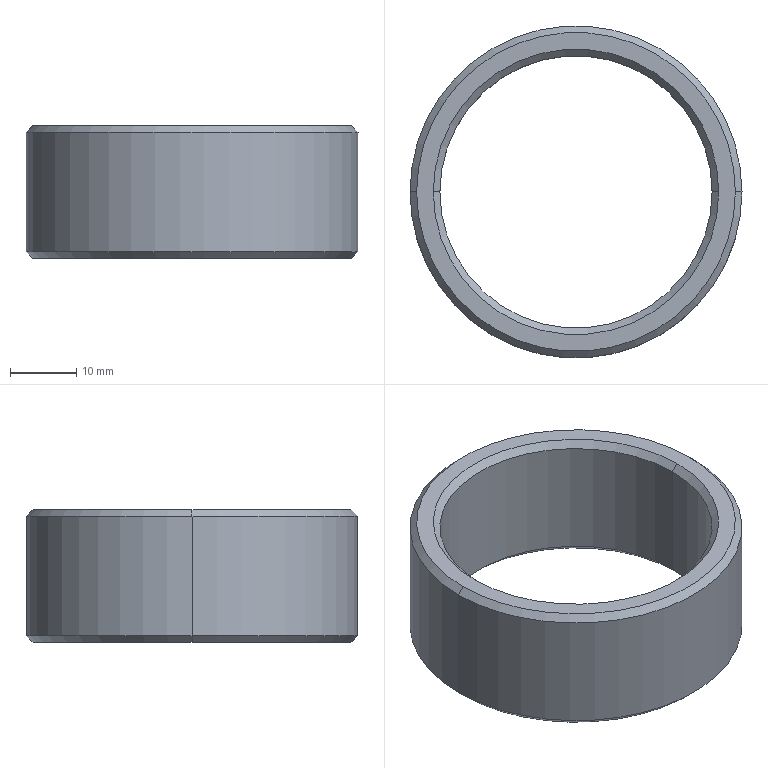Part | STEP file | 1 solid | 14 faces | box 50 x 50 x 20 mm | volume 12579 mm3 | cone 8 | cylinder 4 | plane 2 | commonest cylinder face diameters 41 x2 50 x2
STEP:
#1=CARTESIAN_POINT('',(0.,0.,0.));
#2=DIRECTION('',(0.,0.,1.));
#3=DIRECTION('',(1.,0.,0.));
#4=AXIS2_PLACEMENT_3D('',#1,#2,#3);
#5=CARTESIAN_POINT('',(-20.5,0.,1.));
#6=VERTEX_POINT('',#5);
#7=CARTESIAN_POINT('',(20.5,0.,1.));
#8=VERTEX_POINT('',#7);
#9=CARTESIAN_POINT('',(0.,0.,1.));
#10=DIRECTION('',(0.,0.,-1.));
#11=DIRECTION('',(-1.,0.,0.));
#12=AXIS2_PLACEMENT_3D('',#9,#10,#11);
#13=CIRCLE('',#12,20.5);
#14=CARTESIAN_POINT('',(0.,0.,20.));
#15=DIRECTION('',(0.,0.,-1.));
#16=DIRECTION('',(-1.,0.,0.));
#17=AXIS2_PLACEMENT_3D('',#14,#15,#16);
#18=CYLINDRICAL_SURFACE('',#17,20.5);
#19=CARTESIAN_POINT('',(0.,19.));
#20=DIRECTION('',(1.,0.));
#21=VECTOR('',#20,1.);
#22=LINE('',#19,#21);
#23=(GEOMETRIC_REPRESENTATION_CONTEXT(2)PARAMETRIC_REPRESENTATION_CONTEXT()REPRESENTATION_CONTEXT('',''));
#24=DEFINITIONAL_REPRESENTATION('',(#22),#23);
#25=PCURVE('',#18,#24);
#26=CARTESIAN_POINT('',(0.,0.,0.));
#27=DIRECTION('',(0.,0.,-1.));
#28=DIRECTION('',(-1.,0.,0.));
#29=AXIS2_PLACEMENT_3D('',#26,#27,#28);
#30=CONICAL_SURFACE('',#29,21.5,0.7854);
#31=CARTESIAN_POINT('',(0.,-1.));
#32=DIRECTION('',(1.,0.));
#33=VECTOR('',#32,1.);
#34=LINE('',#31,#33);
#35=(GEOMETRIC_REPRESENTATION_CONTEXT(2)PARAMETRIC_REPRESENTATION_CONTEXT()REPRESENTATION_CONTEXT('',''));
#36=DEFINITIONAL_REPRESENTATION('',(#34),#35);
#37=PCURVE('',#30,#36);
#38=SURFACE_CURVE('',#13,(#25,#37),.PCURVE_S1.);
#39=EDGE_CURVE('',#6,#8,#38,.T.);
#40=ORIENTED_EDGE('',*,*,#39,.F.);
#41=CARTESIAN_POINT('',(-20.5,0.,19.));
#42=VERTEX_POINT('',#41);
#43=CARTESIAN_POINT('',(-20.5,0.,20.));
#44=DIRECTION('',(0.,0.,-1.));
#45=VECTOR('',#44,1.);
#46=LINE('',#43,#45);
#47=CARTESIAN_POINT('',(0.,0.));
#48=DIRECTION('',(0.,1.));
#49=VECTOR('',#48,1.);
#50=LINE('',#47,#49);
#51=(GEOMETRIC_REPRESENTATION_CONTEXT(2)PARAMETRIC_REPRESENTATION_CONTEXT()REPRESENTATION_CONTEXT('',''));
#52=DEFINITIONAL_REPRESENTATION('',(#50),#51);
#53=PCURVE('',#18,#52);
#54=CARTESIAN_POINT('',(0.,0.,20.));
#55=DIRECTION('',(0.,0.,-1.));
#56=DIRECTION('',(-1.,0.,0.));
#57=AXIS2_PLACEMENT_3D('',#54,#55,#56);
#58=CYLINDRICAL_SURFACE('',#57,20.5);
#59=CARTESIAN_POINT('',(6.283,0.));
#60=DIRECTION('',(0.,1.));
#61=VECTOR('',#60,1.);
#62=LINE('',#59,#61);
#63=(GEOMETRIC_REPRESENTATION_CONTEXT(2)PARAMETRIC_REPRESENTATION_CONTEXT()REPRESENTATION_CONTEXT('',''));
#64=DEFINITIONAL_REPRESENTATION('',(#62),#63);
#65=PCURVE('',#58,#64);
#66=SURFACE_CURVE('',#46,(#53,#65),.PCURVE_S1.);
#67=EDGE_CURVE('',#42,#6,#66,.T.);
#68=ORIENTED_EDGE('',*,*,#67,.F.);
#69=CARTESIAN_POINT('',(20.5,0.,19.));
#70=VERTEX_POINT('',#69);
#71=CARTESIAN_POINT('',(0.,0.,19.));
#72=DIRECTION('',(0.,0.,1.));
#73=DIRECTION('',(1.,0.,0.));
#74=AXIS2_PLACEMENT_3D('',#71,#72,#73);
#75=CIRCLE('',#74,20.5);
#76=CARTESIAN_POINT('',(3.142,1.));
#77=DIRECTION('',(-1.,0.));
#78=VECTOR('',#77,1.);
#79=LINE('',#76,#78);
#80=(GEOMETRIC_REPRESENTATION_CONTEXT(2)PARAMETRIC_REPRESENTATION_CONTEXT()REPRESENTATION_CONTEXT('',''));
#81=DEFINITIONAL_REPRESENTATION('',(#79),#80);
#82=PCURVE('',#18,#81);
#83=CARTESIAN_POINT('',(0.,0.,20.));
#84=DIRECTION('',(0.,0.,1.));
#85=DIRECTION('',(1.,0.,0.));
#86=AXIS2_PLACEMENT_3D('',#83,#84,#85);
#87=CONICAL_SURFACE('',#86,21.5,0.7854);
#88=CARTESIAN_POINT('',(0.,-1.));
#89=DIRECTION('',(1.,0.));
#90=VECTOR('',#89,1.);
#91=LINE('',#88,#90);
#92=(GEOMETRIC_REPRESENTATION_CONTEXT(2)PARAMETRIC_REPRESENTATION_CONTEXT()REPRESENTATION_CONTEXT('',''));
#93=DEFINITIONAL_REPRESENTATION('',(#91),#92);
#94=PCURVE('',#87,#93);
#95=SURFACE_CURVE('',#75,(#82,#94),.PCURVE_S1.);
#96=EDGE_CURVE('',#70,#42,#95,.T.);
#97=ORIENTED_EDGE('',*,*,#96,.F.);
#98=CARTESIAN_POINT('',(20.5,0.,20.));
#99=DIRECTION('',(0.,0.,-1.));
#100=VECTOR('',#99,1.);
#101=LINE('',#98,#100);
#102=CARTESIAN_POINT('',(3.142,0.));
#103=DIRECTION('',(0.,1.));
#104=VECTOR('',#103,1.);
#105=LINE('',#102,#104);
#106=(GEOMETRIC_REPRESENTATION_CONTEXT(2)PARAMETRIC_REPRESENTATION_CONTEXT()REPRESENTATION_CONTEXT('',''));
#107=DEFINITIONAL_REPRESENTATION('',(#105),#106);
#108=PCURVE('',#18,#107);
#109=CARTESIAN_POINT('',(3.142,0.));
#110=DIRECTION('',(0.,1.));
#111=VECTOR('',#110,1.);
#112=LINE('',#109,#111);
#113=(GEOMETRIC_REPRESENTATION_CONTEXT(2)PARAMETRIC_REPRESENTATION_CONTEXT()REPRESENTATION_CONTEXT('',''));
#114=DEFINITIONAL_REPRESENTATION('',(#112),#113);
#115=PCURVE('',#58,#114);
#116=SURFACE_CURVE('',#101,(#108,#115),.PCURVE_S1.);
#117=EDGE_CURVE('',#70,#8,#116,.T.);
#118=ORIENTED_EDGE('',*,*,#117,.T.);
#119=EDGE_LOOP('',(#40,#68,#97,#118));
#120=FACE_BOUND('',#119,.F.);
#121=ADVANCED_FACE('',(#120),#18,.F.);
#122=CARTESIAN_POINT('',(-21.5,0.,20.));
#123=VERTEX_POINT('',#122);
#124=CARTESIAN_POINT('',(21.5,0.,20.));
#125=VERTEX_POINT('',#124);
#126=CARTESIAN_POINT('',(0.,0.,20.));
#127=DIRECTION('',(0.,0.,-1.));
#128=DIRECTION('',(1.,0.,0.));
#129=AXIS2_PLACEMENT_3D('',#126,#127,#128);
#130=CIRCLE('',#129,21.5);
#131=CARTESIAN_POINT('',(6.283,0.));
#132=DIRECTION('',(-1.,0.));
#133=VECTOR('',#132,1.);
#134=LINE('',#131,#133);
#135=(GEOMETRIC_REPRESENTATION_CONTEXT(2)PARAMETRIC_REPRESENTATION_CONTEXT()REPRESENTATION_CONTEXT('',''));
#136=DEFINITIONAL_REPRESENTATION('',(#134),#135);
#137=PCURVE('',#87,#136);
#138=CARTESIAN_POINT('',(0.,0.,20.));
#139=DIRECTION('',(0.,0.,1.));
#140=DIRECTION('',(1.,0.,0.));
#141=AXIS2_PLACEMENT_3D('',#138,#139,#140);
#142=PLANE('',#141);
#143=CARTESIAN_POINT('',(21.5,0.));
#144=CARTESIAN_POINT('',(21.5,-37.239));
#145=CARTESIAN_POINT('',(-10.75,-18.62));
#146=CARTESIAN_POINT('',(-43.,0.));
#147=CARTESIAN_POINT('',(-10.75,18.62));
#148=CARTESIAN_POINT('',(21.5,37.239));
#149=CARTESIAN_POINT('',(21.5,0.));
#150=(BOUNDED_CURVE()B_SPLINE_CURVE(2,(#143,#144,#145,#146,#147,#148,#149),.UNSPECIFIED.,.T.,.F.)B_SPLINE_CURVE_WITH_KNOTS((1,2,2,2,2,1),(-2.094,0.,2.094,4.189,6.283,8.378),.UNSPECIFIED.)CURVE()GEOMETRIC_REPRESENTATION_ITEM()RATIONAL_B_SPLINE_CURVE((1.,0.5,1.,0.5,1.,0.5,1.))REPRESENTATION_ITEM(''));
#151=(GEOMETRIC_REPRESENTATION_CONTEXT(2)PARAMETRIC_REPRESENTATION_CONTEXT()REPRESENTATION_CONTEXT('',''));
#152=DEFINITIONAL_REPRESENTATION('',(#150),#151);
#153=PCURVE('',#142,#152);
#154=SURFACE_CURVE('',#130,(#137,#153),.PCURVE_S1.);
#155=EDGE_CURVE('',#123,#125,#154,.T.);
#156=ORIENTED_EDGE('',*,*,#155,.T.);
#157=CARTESIAN_POINT('',(21.5,0.,20.));
#158=DIRECTION('',(0.7071,0.,0.7071));
#159=VECTOR('',#158,1.);
#160=LINE('',#157,#159);
#161=CARTESIAN_POINT('',(0.,0.));
#162=DIRECTION('',(0.,1.));
#163=VECTOR('',#162,1.);
#164=LINE('',#161,#163);
#165=(GEOMETRIC_REPRESENTATION_CONTEXT(2)PARAMETRIC_REPRESENTATION_CONTEXT()REPRESENTATION_CONTEXT('',''));
#166=DEFINITIONAL_REPRESENTATION('',(#164),#165);
#167=PCURVE('',#87,#166);
#168=CARTESIAN_POINT('',(0.,0.,20.));
#169=DIRECTION('',(0.,0.,1.));
#170=DIRECTION('',(1.,0.,0.));
#171=AXIS2_PLACEMENT_3D('',#168,#169,#170);
#172=CONICAL_SURFACE('',#171,21.5,0.7854);
#173=CARTESIAN_POINT('',(6.283,0.));
#174=DIRECTION('',(0.,1.));
#175=VECTOR('',#174,1.);
#176=LINE('',#173,#175);
#177=(GEOMETRIC_REPRESENTATION_CONTEXT(2)PARAMETRIC_REPRESENTATION_CONTEXT()REPRESENTATION_CONTEXT('',''));
#178=DEFINITIONAL_REPRESENTATION('',(#176),#177);
#179=PCURVE('',#172,#178);
#180=SURFACE_CURVE('',#160,(#167,#179),.PCURVE_S1.);
#181=EDGE_CURVE('',#70,#125,#180,.T.);
#182=ORIENTED_EDGE('',*,*,#181,.F.);
#183=ORIENTED_EDGE('',*,*,#96,.T.);
#184=CARTESIAN_POINT('',(-21.5,0.,20.));
#185=DIRECTION('',(-0.7071,0.,0.7071));
#186=VECTOR('',#185,1.);
#187=LINE('',#184,#186);
#188=CARTESIAN_POINT('',(3.142,0.));
#189=DIRECTION('',(0.,1.));
#190=VECTOR('',#189,1.);
#191=LINE('',#188,#190);
#192=(GEOMETRIC_REPRESENTATION_CONTEXT(2)PARAMETRIC_REPRESENTATION_CONTEXT()REPRESENTATION_CONTEXT('',''));
#193=DEFINITIONAL_REPRESENTATION('',(#191),#192);
#194=PCURVE('',#87,#193);
#195=CARTESIAN_POINT('',(3.142,0.));
#196=DIRECTION('',(0.,1.));
#197=VECTOR('',#196,1.);
#198=LINE('',#195,#197);
#199=(GEOMETRIC_REPRESENTATION_CONTEXT(2)PARAMETRIC_REPRESENTATION_CONTEXT()REPRESENTATION_CONTEXT('',''));
#200=DEFINITIONAL_REPRESENTATION('',(#198),#199);
#201=PCURVE('',#172,#200);
#202=SURFACE_CURVE('',#187,(#194,#201),.PCURVE_S1.);
#203=EDGE_CURVE('',#42,#123,#202,.T.);
#204=ORIENTED_EDGE('',*,*,#203,.T.);
#205=EDGE_LOOP('',(#156,#182,#183,#204));
#206=FACE_BOUND('',#205,.F.);
#207=ADVANCED_FACE('',(#206),#87,.F.);
#208=CARTESIAN_POINT('',(-21.5,0.,0.));
#209=VERTEX_POINT('',#208);
#210=CARTESIAN_POINT('',(21.5,0.,0.));
#211=VERTEX_POINT('',#210);
#212=CARTESIAN_POINT('',(0.,0.,0.));
#213=DIRECTION('',(0.,0.,-1.));
#214=DIRECTION('',(-1.,0.,0.));
#215=AXIS2_PLACEMENT_3D('',#212,#213,#214);
#216=CIRCLE('',#215,21.5);
#217=CARTESIAN_POINT('',(0.,0.));
#218=DIRECTION('',(1.,0.));
#219=VECTOR('',#218,1.);
#220=LINE('',#217,#219);
#221=(GEOMETRIC_REPRESENTATION_CONTEXT(2)PARAMETRIC_REPRESENTATION_CONTEXT()REPRESENTATION_CONTEXT('',''));
#222=DEFINITIONAL_REPRESENTATION('',(#220),#221);
#223=PCURVE('',#30,#222);
#224=CARTESIAN_POINT('',(0.,0.,0.));
#225=DIRECTION('',(0.,0.,1.));
#226=DIRECTION('',(1.,0.,0.));
#227=AXIS2_PLACEMENT_3D('',#224,#225,#226);
#228=PLANE('',#227);
#229=CARTESIAN_POINT('',(-21.5,0.));
#230=CARTESIAN_POINT('',(-21.5,37.239));
#231=CARTESIAN_POINT('',(10.75,18.62));
#232=CARTESIAN_POINT('',(43.,0.));
#233=CARTESIAN_POINT('',(10.75,-18.62));
#234=CARTESIAN_POINT('',(-21.5,-37.239));
#235=CARTESIAN_POINT('',(-21.5,0.));
#236=(BOUNDED_CURVE()B_SPLINE_CURVE(2,(#229,#230,#231,#232,#233,#234,#235),.UNSPECIFIED.,.T.,.F.)B_SPLINE_CURVE_WITH_KNOTS((1,2,2,2,2,1),(-2.094,0.,2.094,4.189,6.283,8.378),.UNSPECIFIED.)CURVE()GEOMETRIC_REPRESENTATION_ITEM()RATIONAL_B_SPLINE_CURVE((1.,0.5,1.,0.5,1.,0.5,1.))REPRESENTATION_ITEM(''));
#237=(GEOMETRIC_REPRESENTATION_CONTEXT(2)PARAMETRIC_REPRESENTATION_CONTEXT()REPRESENTATION_CONTEXT('',''));
#238=DEFINITIONAL_REPRESENTATION('',(#236),#237);
#239=PCURVE('',#228,#238);
#240=SURFACE_CURVE('',#216,(#223,#239),.PCURVE_S1.);
#241=EDGE_CURVE('',#209,#211,#240,.T.);
#242=ORIENTED_EDGE('',*,*,#241,.F.);
#243=CARTESIAN_POINT('',(-21.5,0.,0.));
#244=DIRECTION('',(-0.7071,0.,-0.7071));
#245=VECTOR('',#244,1.);
#246=LINE('',#243,#245);
#247=CARTESIAN_POINT('',(0.,0.));
#248=DIRECTION('',(0.,1.));
#249=VECTOR('',#248,1.);
#250=LINE('',#247,#249);
#251=(GEOMETRIC_REPRESENTATION_CONTEXT(2)PARAMETRIC_REPRESENTATION_CONTEXT()REPRESENTATION_CONTEXT('',''));
#252=DEFINITIONAL_REPRESENTATION('',(#250),#251);
#253=PCURVE('',#30,#252);
#254=CARTESIAN_POINT('',(0.,0.,0.));
#255=DIRECTION('',(0.,0.,-1.));
#256=DIRECTION('',(-1.,0.,0.));
#257=AXIS2_PLACEMENT_3D('',#254,#255,#256);
#258=CONICAL_SURFACE('',#257,21.5,0.7854);
#259=CARTESIAN_POINT('',(6.283,0.));
#260=DIRECTION('',(0.,1.));
#261=VECTOR('',#260,1.);
#262=LINE('',#259,#261);
#263=(GEOMETRIC_REPRESENTATION_CONTEXT(2)PARAMETRIC_REPRESENTATION_CONTEXT()REPRESENTATION_CONTEXT('',''));
#264=DEFINITIONAL_REPRESENTATION('',(#262),#263);
#265=PCURVE('',#258,#264);
#266=SURFACE_CURVE('',#246,(#253,#265),.PCURVE_S1.);
#267=EDGE_CURVE('',#6,#209,#266,.T.);
#268=ORIENTED_EDGE('',*,*,#267,.F.);
#269=ORIENTED_EDGE('',*,*,#39,.T.);
#270=CARTESIAN_POINT('',(21.5,0.,0.));
#271=DIRECTION('',(0.7071,0.,-0.7071));
#272=VECTOR('',#271,1.);
#273=LINE('',#270,#272);
#274=CARTESIAN_POINT('',(3.142,0.));
#275=DIRECTION('',(0.,1.));
#276=VECTOR('',#275,1.);
#277=LINE('',#274,#276);
#278=(GEOMETRIC_REPRESENTATION_CONTEXT(2)PARAMETRIC_REPRESENTATION_CONTEXT()REPRESENTATION_CONTEXT('',''));
#279=DEFINITIONAL_REPRESENTATION('',(#277),#278);
#280=PCURVE('',#30,#279);
#281=CARTESIAN_POINT('',(3.142,0.));
#282=DIRECTION('',(0.,1.));
#283=VECTOR('',#282,1.);
#284=LINE('',#281,#283);
#285=(GEOMETRIC_REPRESENTATION_CONTEXT(2)PARAMETRIC_REPRESENTATION_CONTEXT()REPRESENTATION_CONTEXT('',''));
#286=DEFINITIONAL_REPRESENTATION('',(#284),#285);
#287=PCURVE('',#258,#286);
#288=SURFACE_CURVE('',#273,(#280,#287),.PCURVE_S1.);
#289=EDGE_CURVE('',#8,#211,#288,.T.);
#290=ORIENTED_EDGE('',*,*,#289,.T.);
#291=EDGE_LOOP('',(#242,#268,#269,#290));
#292=FACE_BOUND('',#291,.F.);
#293=ADVANCED_FACE('',(#292),#30,.F.);
#294=CARTESIAN_POINT('',(0.,0.,20.));
#295=DIRECTION('',(0.,0.,-1.));
#296=DIRECTION('',(1.,0.,0.));
#297=AXIS2_PLACEMENT_3D('',#294,#295,#296);
#298=CIRCLE('',#297,21.5);
#299=CARTESIAN_POINT('',(21.5,0.));
#300=CARTESIAN_POINT('',(21.5,-37.239));
#301=CARTESIAN_POINT('',(-10.75,-18.62));
#302=CARTESIAN_POINT('',(-43.,0.));
#303=CARTESIAN_POINT('',(-10.75,18.62));
#304=CARTESIAN_POINT('',(21.5,37.239));
#305=CARTESIAN_POINT('',(21.5,0.));
#306=(BOUNDED_CURVE()B_SPLINE_CURVE(2,(#299,#300,#301,#302,#303,#304,#305),.UNSPECIFIED.,.T.,.F.)B_SPLINE_CURVE_WITH_KNOTS((1,2,2,2,2,1),(-2.094,0.,2.094,4.189,6.283,8.378),.UNSPECIFIED.)CURVE()GEOMETRIC_REPRESENTATION_ITEM()RATIONAL_B_SPLINE_CURVE((1.,0.5,1.,0.5,1.,0.5,1.))REPRESENTATION_ITEM(''));
#307=(GEOMETRIC_REPRESENTATION_CONTEXT(2)PARAMETRIC_REPRESENTATION_CONTEXT()REPRESENTATION_CONTEXT('',''));
#308=DEFINITIONAL_REPRESENTATION('',(#306),#307);
#309=PCURVE('',#142,#308);
#310=CARTESIAN_POINT('',(6.283,0.));
#311=DIRECTION('',(-1.,0.));
#312=VECTOR('',#311,1.);
#313=LINE('',#310,#312);
#314=(GEOMETRIC_REPRESENTATION_CONTEXT(2)PARAMETRIC_REPRESENTATION_CONTEXT()REPRESENTATION_CONTEXT('',''));
#315=DEFINITIONAL_REPRESENTATION('',(#313),#314);
#316=PCURVE('',#172,#315);
#317=SURFACE_CURVE('',#298,(#309,#316),.PCURVE_S1.);
#318=EDGE_CURVE('',#125,#123,#317,.T.);
#319=ORIENTED_EDGE('',*,*,#318,.T.);
#320=ORIENTED_EDGE('',*,*,#155,.T.);
#321=EDGE_LOOP('',(#319,#320));
#322=FACE_BOUND('',#321,.T.);
#323=CARTESIAN_POINT('',(-24.,0.,20.));
#324=VERTEX_POINT('',#323);
#325=CARTESIAN_POINT('',(24.,0.,20.));
#326=VERTEX_POINT('',#325);
#327=CARTESIAN_POINT('',(0.,0.,20.));
#328=DIRECTION('',(0.,0.,-1.));
#329=DIRECTION('',(-1.,0.,0.));
#330=AXIS2_PLACEMENT_3D('',#327,#328,#329);
#331=CIRCLE('',#330,24.);
#332=CARTESIAN_POINT('',(-24.,0.));
#333=CARTESIAN_POINT('',(-24.,41.569));
#334=CARTESIAN_POINT('',(12.,20.785));
#335=CARTESIAN_POINT('',(48.,0.));
#336=CARTESIAN_POINT('',(12.,-20.785));
#337=CARTESIAN_POINT('',(-24.,-41.569));
#338=CARTESIAN_POINT('',(-24.,0.));
#339=(BOUNDED_CURVE()B_SPLINE_CURVE(2,(#332,#333,#334,#335,#336,#337,#338),.UNSPECIFIED.,.T.,.F.)B_SPLINE_CURVE_WITH_KNOTS((1,2,2,2,2,1),(-2.094,0.,2.094,4.189,6.283,8.378),.UNSPECIFIED.)CURVE()GEOMETRIC_REPRESENTATION_ITEM()RATIONAL_B_SPLINE_CURVE((1.,0.5,1.,0.5,1.,0.5,1.))REPRESENTATION_ITEM(''));
#340=(GEOMETRIC_REPRESENTATION_CONTEXT(2)PARAMETRIC_REPRESENTATION_CONTEXT()REPRESENTATION_CONTEXT('',''));
#341=DEFINITIONAL_REPRESENTATION('',(#339),#340);
#342=PCURVE('',#142,#341);
#343=CARTESIAN_POINT('',(0.,0.,19.));
#344=DIRECTION('',(0.,0.,-1.));
#345=DIRECTION('',(-1.,0.,0.));
#346=AXIS2_PLACEMENT_3D('',#343,#344,#345);
#347=CONICAL_SURFACE('',#346,25.,0.7854);
#348=CARTESIAN_POINT('',(0.,-1.));
#349=DIRECTION('',(1.,0.));
#350=VECTOR('',#349,1.);
#351=LINE('',#348,#350);
#352=(GEOMETRIC_REPRESENTATION_CONTEXT(2)PARAMETRIC_REPRESENTATION_CONTEXT()REPRESENTATION_CONTEXT('',''));
#353=DEFINITIONAL_REPRESENTATION('',(#351),#352);
#354=PCURVE('',#347,#353);
#355=SURFACE_CURVE('',#331,(#342,#354),.PCURVE_S1.);
#356=EDGE_CURVE('',#324,#326,#355,.T.);
#357=ORIENTED_EDGE('',*,*,#356,.F.);
#358=CARTESIAN_POINT('',(0.,0.,20.));
#359=DIRECTION('',(0.,0.,-1.));
#360=DIRECTION('',(-1.,0.,0.));
#361=AXIS2_PLACEMENT_3D('',#358,#359,#360);
#362=CIRCLE('',#361,24.);
#363=CARTESIAN_POINT('',(-24.,0.));
#364=CARTESIAN_POINT('',(-24.,41.569));
#365=CARTESIAN_POINT('',(12.,20.785));
#366=CARTESIAN_POINT('',(48.,0.));
#367=CARTESIAN_POINT('',(12.,-20.785));
#368=CARTESIAN_POINT('',(-24.,-41.569));
#369=CARTESIAN_POINT('',(-24.,0.));
#370=(BOUNDED_CURVE()B_SPLINE_CURVE(2,(#363,#364,#365,#366,#367,#368,#369),.UNSPECIFIED.,.T.,.F.)B_SPLINE_CURVE_WITH_KNOTS((1,2,2,2,2,1),(-2.094,0.,2.094,4.189,6.283,8.378),.UNSPECIFIED.)CURVE()GEOMETRIC_REPRESENTATION_ITEM()RATIONAL_B_SPLINE_CURVE((1.,0.5,1.,0.5,1.,0.5,1.))REPRESENTATION_ITEM(''));
#371=(GEOMETRIC_REPRESENTATION_CONTEXT(2)PARAMETRIC_REPRESENTATION_CONTEXT()REPRESENTATION_CONTEXT('',''));
#372=DEFINITIONAL_REPRESENTATION('',(#370),#371);
#373=PCURVE('',#142,#372);
#374=CARTESIAN_POINT('',(0.,0.,19.));
#375=DIRECTION('',(0.,0.,-1.));
#376=DIRECTION('',(-1.,0.,0.));
#377=AXIS2_PLACEMENT_3D('',#374,#375,#376);
#378=CONICAL_SURFACE('',#377,25.,0.7854);
#379=CARTESIAN_POINT('',(0.,-1.));
#380=DIRECTION('',(1.,0.));
#381=VECTOR('',#380,1.);
#382=LINE('',#379,#381);
#383=(GEOMETRIC_REPRESENTATION_CONTEXT(2)PARAMETRIC_REPRESENTATION_CONTEXT()REPRESENTATION_CONTEXT('',''));
#384=DEFINITIONAL_REPRESENTATION('',(#382),#383);
#385=PCURVE('',#378,#384);
#386=SURFACE_CURVE('',#362,(#373,#385),.PCURVE_S1.);
#387=EDGE_CURVE('',#326,#324,#386,.T.);
#388=ORIENTED_EDGE('',*,*,#387,.F.);
#389=EDGE_LOOP('',(#357,#388));
#390=FACE_BOUND('',#389,.T.);
#391=ADVANCED_FACE('',(#322,#390),#142,.T.);
#392=ORIENTED_EDGE('',*,*,#241,.F.);
#393=CARTESIAN_POINT('',(0.,0.,0.));
#394=DIRECTION('',(0.,0.,-1.));
#395=DIRECTION('',(-1.,0.,0.));
#396=AXIS2_PLACEMENT_3D('',#393,#394,#395);
#397=CIRCLE('',#396,21.5);
#398=CARTESIAN_POINT('',(-21.5,0.));
#399=CARTESIAN_POINT('',(-21.5,37.239));
#400=CARTESIAN_POINT('',(10.75,18.62));
#401=CARTESIAN_POINT('',(43.,0.));
#402=CARTESIAN_POINT('',(10.75,-18.62));
#403=CARTESIAN_POINT('',(-21.5,-37.239));
#404=CARTESIAN_POINT('',(-21.5,0.));
#405=(BOUNDED_CURVE()B_SPLINE_CURVE(2,(#398,#399,#400,#401,#402,#403,#404),.UNSPECIFIED.,.T.,.F.)B_SPLINE_CURVE_WITH_KNOTS((1,2,2,2,2,1),(-2.094,0.,2.094,4.189,6.283,8.378),.UNSPECIFIED.)CURVE()GEOMETRIC_REPRESENTATION_ITEM()RATIONAL_B_SPLINE_CURVE((1.,0.5,1.,0.5,1.,0.5,1.))REPRESENTATION_ITEM(''));
#406=(GEOMETRIC_REPRESENTATION_CONTEXT(2)PARAMETRIC_REPRESENTATION_CONTEXT()REPRESENTATION_CONTEXT('',''));
#407=DEFINITIONAL_REPRESENTATION('',(#405),#406);
#408=PCURVE('',#228,#407);
#409=CARTESIAN_POINT('',(0.,0.));
#410=DIRECTION('',(1.,0.));
#411=VECTOR('',#410,1.);
#412=LINE('',#409,#411);
#413=(GEOMETRIC_REPRESENTATION_CONTEXT(2)PARAMETRIC_REPRESENTATION_CONTEXT()REPRESENTATION_CONTEXT('',''));
#414=DEFINITIONAL_REPRESENTATION('',(#412),#413);
#415=PCURVE('',#258,#414);
#416=SURFACE_CURVE('',#397,(#408,#415),.PCURVE_S1.);
#417=EDGE_CURVE('',#211,#209,#416,.T.);
#418=ORIENTED_EDGE('',*,*,#417,.F.);
#419=EDGE_LOOP('',(#392,#418));
#420=FACE_BOUND('',#419,.T.);
#421=CARTESIAN_POINT('',(24.,0.,0.));
#422=VERTEX_POINT('',#421);
#423=CARTESIAN_POINT('',(-24.,0.,0.));
#424=VERTEX_POINT('',#423);
#425=CARTESIAN_POINT('',(0.,0.,0.));
#426=DIRECTION('',(0.,0.,1.));
#427=DIRECTION('',(1.,0.,0.));
#428=AXIS2_PLACEMENT_3D('',#425,#426,#427);
#429=CIRCLE('',#428,24.);
#430=CARTESIAN_POINT('',(0.,0.));
#431=DIRECTION('',(1.,0.));
#432=AXIS2_PLACEMENT_2D('',#430,#431);
#433=CIRCLE('',#432,24.);
#434=(GEOMETRIC_REPRESENTATION_CONTEXT(2)PARAMETRIC_REPRESENTATION_CONTEXT()REPRESENTATION_CONTEXT('',''));
#435=DEFINITIONAL_REPRESENTATION('',(#433),#434);
#436=PCURVE('',#228,#435);
#437=CARTESIAN_POINT('',(0.,0.,1.));
#438=DIRECTION('',(0.,0.,1.));
#439=DIRECTION('',(1.,0.,0.));
#440=AXIS2_PLACEMENT_3D('',#437,#438,#439);
#441=CONICAL_SURFACE('',#440,25.,0.7854);
#442=CARTESIAN_POINT('',(0.,-1.));
#443=DIRECTION('',(1.,0.));
#444=VECTOR('',#443,1.);
#445=LINE('',#442,#444);
#446=(GEOMETRIC_REPRESENTATION_CONTEXT(2)PARAMETRIC_REPRESENTATION_CONTEXT()REPRESENTATION_CONTEXT('',''));
#447=DEFINITIONAL_REPRESENTATION('',(#445),#446);
#448=PCURVE('',#441,#447);
#449=SURFACE_CURVE('',#429,(#436,#448),.PCURVE_S1.);
#450=EDGE_CURVE('',#422,#424,#449,.T.);
#451=ORIENTED_EDGE('',*,*,#450,.F.);
#452=CARTESIAN_POINT('',(0.,0.,0.));
#453=DIRECTION('',(0.,0.,1.));
#454=DIRECTION('',(1.,0.,0.));
#455=AXIS2_PLACEMENT_3D('',#452,#453,#454);
#456=CIRCLE('',#455,24.);
#457=CARTESIAN_POINT('',(0.,0.));
#458=DIRECTION('',(1.,0.));
#459=AXIS2_PLACEMENT_2D('',#457,#458);
#460=CIRCLE('',#459,24.);
#461=(GEOMETRIC_REPRESENTATION_CONTEXT(2)PARAMETRIC_REPRESENTATION_CONTEXT()REPRESENTATION_CONTEXT('',''));
#462=DEFINITIONAL_REPRESENTATION('',(#460),#461);
#463=PCURVE('',#228,#462);
#464=CARTESIAN_POINT('',(0.,0.,1.));
#465=DIRECTION('',(0.,0.,1.));
#466=DIRECTION('',(1.,0.,0.));
#467=AXIS2_PLACEMENT_3D('',#464,#465,#466);
#468=CONICAL_SURFACE('',#467,25.,0.7854);
#469=CARTESIAN_POINT('',(0.,-1.));
#470=DIRECTION('',(1.,0.));
#471=VECTOR('',#470,1.);
#472=LINE('',#469,#471);
#473=(GEOMETRIC_REPRESENTATION_CONTEXT(2)PARAMETRIC_REPRESENTATION_CONTEXT()REPRESENTATION_CONTEXT('',''));
#474=DEFINITIONAL_REPRESENTATION('',(#472),#473);
#475=PCURVE('',#468,#474);
#476=SURFACE_CURVE('',#456,(#463,#475),.PCURVE_S1.);
#477=EDGE_CURVE('',#424,#422,#476,.T.);
#478=ORIENTED_EDGE('',*,*,#477,.F.);
#479=EDGE_LOOP('',(#451,#478));
#480=FACE_BOUND('',#479,.T.);
#481=ADVANCED_FACE('',(#420,#480),#228,.F.);
#482=CARTESIAN_POINT('',(25.,0.,19.));
#483=VERTEX_POINT('',#482);
#484=CARTESIAN_POINT('',(25.,0.,19.));
#485=DIRECTION('',(0.7071,0.,-0.7071));
#486=VECTOR('',#485,1.);
#487=LINE('',#484,#486);
#488=CARTESIAN_POINT('',(3.142,0.));
#489=DIRECTION('',(0.,1.));
#490=VECTOR('',#489,1.);
#491=LINE('',#488,#490);
#492=(GEOMETRIC_REPRESENTATION_CONTEXT(2)PARAMETRIC_REPRESENTATION_CONTEXT()REPRESENTATION_CONTEXT('',''));
#493=DEFINITIONAL_REPRESENTATION('',(#491),#492);
#494=PCURVE('',#378,#493);
#495=CARTESIAN_POINT('',(3.142,0.));
#496=DIRECTION('',(0.,1.));
#497=VECTOR('',#496,1.);
#498=LINE('',#495,#497);
#499=(GEOMETRIC_REPRESENTATION_CONTEXT(2)PARAMETRIC_REPRESENTATION_CONTEXT()REPRESENTATION_CONTEXT('',''));
#500=DEFINITIONAL_REPRESENTATION('',(#498),#499);
#501=PCURVE('',#347,#500);
#502=SURFACE_CURVE('',#487,(#494,#501),.PCURVE_S1.);
#503=EDGE_CURVE('',#326,#483,#502,.T.);
#504=ORIENTED_EDGE('',*,*,#503,.F.);
#505=ORIENTED_EDGE('',*,*,#387,.T.);
#506=CARTESIAN_POINT('',(-25.,0.,19.));
#507=VERTEX_POINT('',#506);
#508=CARTESIAN_POINT('',(-25.,0.,19.));
#509=DIRECTION('',(-0.7071,0.,-0.7071));
#510=VECTOR('',#509,1.);
#511=LINE('',#508,#510);
#512=CARTESIAN_POINT('',(6.283,0.));
#513=DIRECTION('',(0.,1.));
#514=VECTOR('',#513,1.);
#515=LINE('',#512,#514);
#516=(GEOMETRIC_REPRESENTATION_CONTEXT(2)PARAMETRIC_REPRESENTATION_CONTEXT()REPRESENTATION_CONTEXT('',''));
#517=DEFINITIONAL_REPRESENTATION('',(#515),#516);
#518=PCURVE('',#378,#517);
#519=CARTESIAN_POINT('',(0.,0.));
#520=DIRECTION('',(0.,1.));
#521=VECTOR('',#520,1.);
#522=LINE('',#519,#521);
#523=(GEOMETRIC_REPRESENTATION_CONTEXT(2)PARAMETRIC_REPRESENTATION_CONTEXT()REPRESENTATION_CONTEXT('',''));
#524=DEFINITIONAL_REPRESENTATION('',(#522),#523);
#525=PCURVE('',#347,#524);
#526=SURFACE_CURVE('',#511,(#518,#525),.PCURVE_S1.);
#527=EDGE_CURVE('',#324,#507,#526,.T.);
#528=ORIENTED_EDGE('',*,*,#527,.T.);
#529=CARTESIAN_POINT('',(0.,0.,19.));
#530=DIRECTION('',(0.,0.,-1.));
#531=DIRECTION('',(-1.,0.,0.));
#532=AXIS2_PLACEMENT_3D('',#529,#530,#531);
#533=CIRCLE('',#532,25.);
#534=CARTESIAN_POINT('',(0.,0.));
#535=DIRECTION('',(1.,0.));
#536=VECTOR('',#535,1.);
#537=LINE('',#534,#536);
#538=(GEOMETRIC_REPRESENTATION_CONTEXT(2)PARAMETRIC_REPRESENTATION_CONTEXT()REPRESENTATION_CONTEXT('',''));
#539=DEFINITIONAL_REPRESENTATION('',(#537),#538);
#540=PCURVE('',#378,#539);
#541=CARTESIAN_POINT('',(0.,0.,20.));
#542=DIRECTION('',(0.,0.,-1.));
#543=DIRECTION('',(-1.,0.,0.));
#544=AXIS2_PLACEMENT_3D('',#541,#542,#543);
#545=CYLINDRICAL_SURFACE('',#544,25.);
#546=CARTESIAN_POINT('',(0.,1.));
#547=DIRECTION('',(1.,0.));
#548=VECTOR('',#547,1.);
#549=LINE('',#546,#548);
#550=(GEOMETRIC_REPRESENTATION_CONTEXT(2)PARAMETRIC_REPRESENTATION_CONTEXT()REPRESENTATION_CONTEXT('',''));
#551=DEFINITIONAL_REPRESENTATION('',(#549),#550);
#552=PCURVE('',#545,#551);
#553=SURFACE_CURVE('',#533,(#540,#552),.PCURVE_S1.);
#554=EDGE_CURVE('',#483,#507,#553,.T.);
#555=ORIENTED_EDGE('',*,*,#554,.F.);
#556=EDGE_LOOP('',(#504,#505,#528,#555));
#557=FACE_BOUND('',#556,.T.);
#558=ADVANCED_FACE('',(#557),#378,.T.);
#559=CARTESIAN_POINT('',(-25.,0.,1.));
#560=VERTEX_POINT('',#559);
#561=CARTESIAN_POINT('',(-25.,0.,1.));
#562=DIRECTION('',(-0.7071,0.,0.7071));
#563=VECTOR('',#562,1.);
#564=LINE('',#561,#563);
#565=CARTESIAN_POINT('',(3.142,0.));
#566=DIRECTION('',(0.,1.));
#567=VECTOR('',#566,1.);
#568=LINE('',#565,#567);
#569=(GEOMETRIC_REPRESENTATION_CONTEXT(2)PARAMETRIC_REPRESENTATION_CONTEXT()REPRESENTATION_CONTEXT('',''));
#570=DEFINITIONAL_REPRESENTATION('',(#568),#569);
#571=PCURVE('',#468,#570);
#572=CARTESIAN_POINT('',(3.142,0.));
#573=DIRECTION('',(0.,1.));
#574=VECTOR('',#573,1.);
#575=LINE('',#572,#574);
#576=(GEOMETRIC_REPRESENTATION_CONTEXT(2)PARAMETRIC_REPRESENTATION_CONTEXT()REPRESENTATION_CONTEXT('',''));
#577=DEFINITIONAL_REPRESENTATION('',(#575),#576);
#578=PCURVE('',#441,#577);
#579=SURFACE_CURVE('',#564,(#571,#578),.PCURVE_S1.);
#580=EDGE_CURVE('',#424,#560,#579,.T.);
#581=ORIENTED_EDGE('',*,*,#580,.F.);
#582=ORIENTED_EDGE('',*,*,#477,.T.);
#583=CARTESIAN_POINT('',(25.,0.,1.));
#584=VERTEX_POINT('',#583);
#585=CARTESIAN_POINT('',(25.,0.,1.));
#586=DIRECTION('',(0.7071,0.,0.7071));
#587=VECTOR('',#586,1.);
#588=LINE('',#585,#587);
#589=CARTESIAN_POINT('',(6.283,0.));
#590=DIRECTION('',(0.,1.));
#591=VECTOR('',#590,1.);
#592=LINE('',#589,#591);
#593=(GEOMETRIC_REPRESENTATION_CONTEXT(2)PARAMETRIC_REPRESENTATION_CONTEXT()REPRESENTATION_CONTEXT('',''));
#594=DEFINITIONAL_REPRESENTATION('',(#592),#593);
#595=PCURVE('',#468,#594);
#596=CARTESIAN_POINT('',(0.,0.));
#597=DIRECTION('',(0.,1.));
#598=VECTOR('',#597,1.);
#599=LINE('',#596,#598);
#600=(GEOMETRIC_REPRESENTATION_CONTEXT(2)PARAMETRIC_REPRESENTATION_CONTEXT()REPRESENTATION_CONTEXT('',''));
#601=DEFINITIONAL_REPRESENTATION('',(#599),#600);
#602=PCURVE('',#441,#601);
#603=SURFACE_CURVE('',#588,(#595,#602),.PCURVE_S1.);
#604=EDGE_CURVE('',#422,#584,#603,.T.);
#605=ORIENTED_EDGE('',*,*,#604,.T.);
#606=CARTESIAN_POINT('',(0.,0.,1.));
#607=DIRECTION('',(0.,0.,1.));
#608=DIRECTION('',(-1.,0.,0.));
#609=AXIS2_PLACEMENT_3D('',#606,#607,#608);
#610=CIRCLE('',#609,25.);
#611=CARTESIAN_POINT('',(3.142,0.));
#612=DIRECTION('',(1.,0.));
#613=VECTOR('',#612,1.);
#614=LINE('',#611,#613);
#615=(GEOMETRIC_REPRESENTATION_CONTEXT(2)PARAMETRIC_REPRESENTATION_CONTEXT()REPRESENTATION_CONTEXT('',''));
#616=DEFINITIONAL_REPRESENTATION('',(#614),#615);
#617=PCURVE('',#468,#616);
#618=CARTESIAN_POINT('',(6.283,19.));
#619=DIRECTION('',(-1.,0.));
#620=VECTOR('',#619,1.);
#621=LINE('',#618,#620);
#622=(GEOMETRIC_REPRESENTATION_CONTEXT(2)PARAMETRIC_REPRESENTATION_CONTEXT()REPRESENTATION_CONTEXT('',''));
#623=DEFINITIONAL_REPRESENTATION('',(#621),#622);
#624=PCURVE('',#545,#623);
#625=SURFACE_CURVE('',#610,(#617,#624),.PCURVE_S1.);
#626=EDGE_CURVE('',#560,#584,#625,.T.);
#627=ORIENTED_EDGE('',*,*,#626,.F.);
#628=EDGE_LOOP('',(#581,#582,#605,#627));
#629=FACE_BOUND('',#628,.T.);
#630=ADVANCED_FACE('',(#629),#468,.T.);
#631=CARTESIAN_POINT('',(25.,0.,20.));
#632=DIRECTION('',(0.,0.,-1.));
#633=VECTOR('',#632,1.);
#634=LINE('',#631,#633);
#635=CARTESIAN_POINT('',(3.142,0.));
#636=DIRECTION('',(0.,1.));
#637=VECTOR('',#636,1.);
#638=LINE('',#635,#637);
#639=(GEOMETRIC_REPRESENTATION_CONTEXT(2)PARAMETRIC_REPRESENTATION_CONTEXT()REPRESENTATION_CONTEXT('',''));
#640=DEFINITIONAL_REPRESENTATION('',(#638),#639);
#641=PCURVE('',#545,#640);
#642=CARTESIAN_POINT('',(0.,0.,20.));
#643=DIRECTION('',(0.,0.,-1.));
#644=DIRECTION('',(-1.,0.,0.));
#645=AXIS2_PLACEMENT_3D('',#642,#643,#644);
#646=CYLINDRICAL_SURFACE('',#645,25.);
#647=CARTESIAN_POINT('',(3.142,0.));
#648=DIRECTION('',(0.,1.));
#649=VECTOR('',#648,1.);
#650=LINE('',#647,#649);
#651=(GEOMETRIC_REPRESENTATION_CONTEXT(2)PARAMETRIC_REPRESENTATION_CONTEXT()REPRESENTATION_CONTEXT('',''));
#652=DEFINITIONAL_REPRESENTATION('',(#650),#651);
#653=PCURVE('',#646,#652);
#654=SURFACE_CURVE('',#634,(#641,#653),.PCURVE_S1.);
#655=EDGE_CURVE('',#483,#584,#654,.T.);
#656=ORIENTED_EDGE('',*,*,#655,.F.);
#657=ORIENTED_EDGE('',*,*,#554,.T.);
#658=CARTESIAN_POINT('',(-25.,0.,20.));
#659=DIRECTION('',(0.,0.,-1.));
#660=VECTOR('',#659,1.);
#661=LINE('',#658,#660);
#662=CARTESIAN_POINT('',(6.283,0.));
#663=DIRECTION('',(0.,1.));
#664=VECTOR('',#663,1.);
#665=LINE('',#662,#664);
#666=(GEOMETRIC_REPRESENTATION_CONTEXT(2)PARAMETRIC_REPRESENTATION_CONTEXT()REPRESENTATION_CONTEXT('',''));
#667=DEFINITIONAL_REPRESENTATION('',(#665),#666);
#668=PCURVE('',#545,#667);
#669=CARTESIAN_POINT('',(0.,0.));
#670=DIRECTION('',(0.,1.));
#671=VECTOR('',#670,1.);
#672=LINE('',#669,#671);
#673=(GEOMETRIC_REPRESENTATION_CONTEXT(2)PARAMETRIC_REPRESENTATION_CONTEXT()REPRESENTATION_CONTEXT('',''));
#674=DEFINITIONAL_REPRESENTATION('',(#672),#673);
#675=PCURVE('',#646,#674);
#676=SURFACE_CURVE('',#661,(#668,#675),.PCURVE_S1.);
#677=EDGE_CURVE('',#507,#560,#676,.T.);
#678=ORIENTED_EDGE('',*,*,#677,.T.);
#679=ORIENTED_EDGE('',*,*,#626,.T.);
#680=EDGE_LOOP('',(#656,#657,#678,#679));
#681=FACE_BOUND('',#680,.T.);
#682=ADVANCED_FACE('',(#681),#545,.T.);
#683=ORIENTED_EDGE('',*,*,#67,.T.);
#684=CARTESIAN_POINT('',(0.,0.,1.));
#685=DIRECTION('',(0.,0.,-1.));
#686=DIRECTION('',(-1.,0.,0.));
#687=AXIS2_PLACEMENT_3D('',#684,#685,#686);
#688=CIRCLE('',#687,20.5);
#689=CARTESIAN_POINT('',(0.,19.));
#690=DIRECTION('',(1.,0.));
#691=VECTOR('',#690,1.);
#692=LINE('',#689,#691);
#693=(GEOMETRIC_REPRESENTATION_CONTEXT(2)PARAMETRIC_REPRESENTATION_CONTEXT()REPRESENTATION_CONTEXT('',''));
#694=DEFINITIONAL_REPRESENTATION('',(#692),#693);
#695=PCURVE('',#58,#694);
#696=CARTESIAN_POINT('',(0.,-1.));
#697=DIRECTION('',(1.,0.));
#698=VECTOR('',#697,1.);
#699=LINE('',#696,#698);
#700=(GEOMETRIC_REPRESENTATION_CONTEXT(2)PARAMETRIC_REPRESENTATION_CONTEXT()REPRESENTATION_CONTEXT('',''));
#701=DEFINITIONAL_REPRESENTATION('',(#699),#700);
#702=PCURVE('',#258,#701);
#703=SURFACE_CURVE('',#688,(#695,#702),.PCURVE_S1.);
#704=EDGE_CURVE('',#8,#6,#703,.T.);
#705=ORIENTED_EDGE('',*,*,#704,.F.);
#706=ORIENTED_EDGE('',*,*,#117,.F.);
#707=CARTESIAN_POINT('',(0.,0.,19.));
#708=DIRECTION('',(0.,0.,1.));
#709=DIRECTION('',(1.,0.,0.));
#710=AXIS2_PLACEMENT_3D('',#707,#708,#709);
#711=CIRCLE('',#710,20.5);
#712=CARTESIAN_POINT('',(9.425,1.));
#713=DIRECTION('',(-1.,0.));
#714=VECTOR('',#713,1.);
#715=LINE('',#712,#714);
#716=(GEOMETRIC_REPRESENTATION_CONTEXT(2)PARAMETRIC_REPRESENTATION_CONTEXT()REPRESENTATION_CONTEXT('',''));
#717=DEFINITIONAL_REPRESENTATION('',(#715),#716);
#718=PCURVE('',#58,#717);
#719=CARTESIAN_POINT('',(0.,-1.));
#720=DIRECTION('',(1.,0.));
#721=VECTOR('',#720,1.);
#722=LINE('',#719,#721);
#723=(GEOMETRIC_REPRESENTATION_CONTEXT(2)PARAMETRIC_REPRESENTATION_CONTEXT()REPRESENTATION_CONTEXT('',''));
#724=DEFINITIONAL_REPRESENTATION('',(#722),#723);
#725=PCURVE('',#172,#724);
#726=SURFACE_CURVE('',#711,(#718,#725),.PCURVE_S1.);
#727=EDGE_CURVE('',#42,#70,#726,.T.);
#728=ORIENTED_EDGE('',*,*,#727,.F.);
#729=EDGE_LOOP('',(#683,#705,#706,#728));
#730=FACE_BOUND('',#729,.F.);
#731=ADVANCED_FACE('',(#730),#58,.F.);
#732=ORIENTED_EDGE('',*,*,#181,.T.);
#733=ORIENTED_EDGE('',*,*,#318,.T.);
#734=ORIENTED_EDGE('',*,*,#203,.F.);
#735=ORIENTED_EDGE('',*,*,#727,.T.);
#736=EDGE_LOOP('',(#732,#733,#734,#735));
#737=FACE_BOUND('',#736,.F.);
#738=ADVANCED_FACE('',(#737),#172,.F.);
#739=ORIENTED_EDGE('',*,*,#267,.T.);
#740=ORIENTED_EDGE('',*,*,#417,.F.);
#741=ORIENTED_EDGE('',*,*,#289,.F.);
#742=ORIENTED_EDGE('',*,*,#704,.T.);
#743=EDGE_LOOP('',(#739,#740,#741,#742));
#744=FACE_BOUND('',#743,.F.);
#745=ADVANCED_FACE('',(#744),#258,.F.);
#746=ORIENTED_EDGE('',*,*,#356,.T.);
#747=ORIENTED_EDGE('',*,*,#503,.T.);
#748=CARTESIAN_POINT('',(0.,0.,19.));
#749=DIRECTION('',(0.,0.,-1.));
#750=DIRECTION('',(-1.,0.,0.));
#751=AXIS2_PLACEMENT_3D('',#748,#749,#750);
#752=CIRCLE('',#751,25.);
#753=CARTESIAN_POINT('',(0.,0.));
#754=DIRECTION('',(1.,0.));
#755=VECTOR('',#754,1.);
#756=LINE('',#753,#755);
#757=(GEOMETRIC_REPRESENTATION_CONTEXT(2)PARAMETRIC_REPRESENTATION_CONTEXT()REPRESENTATION_CONTEXT('',''));
#758=DEFINITIONAL_REPRESENTATION('',(#756),#757);
#759=PCURVE('',#347,#758);
#760=CARTESIAN_POINT('',(0.,1.));
#761=DIRECTION('',(1.,0.));
#762=VECTOR('',#761,1.);
#763=LINE('',#760,#762);
#764=(GEOMETRIC_REPRESENTATION_CONTEXT(2)PARAMETRIC_REPRESENTATION_CONTEXT()REPRESENTATION_CONTEXT('',''));
#765=DEFINITIONAL_REPRESENTATION('',(#763),#764);
#766=PCURVE('',#646,#765);
#767=SURFACE_CURVE('',#752,(#759,#766),.PCURVE_S1.);
#768=EDGE_CURVE('',#507,#483,#767,.T.);
#769=ORIENTED_EDGE('',*,*,#768,.F.);
#770=ORIENTED_EDGE('',*,*,#527,.F.);
#771=EDGE_LOOP('',(#746,#747,#769,#770));
#772=FACE_BOUND('',#771,.T.);
#773=ADVANCED_FACE('',(#772),#347,.T.);
#774=ORIENTED_EDGE('',*,*,#450,.T.);
#775=ORIENTED_EDGE('',*,*,#580,.T.);
#776=CARTESIAN_POINT('',(0.,0.,1.));
#777=DIRECTION('',(0.,0.,1.));
#778=DIRECTION('',(-1.,0.,0.));
#779=AXIS2_PLACEMENT_3D('',#776,#777,#778);
#780=CIRCLE('',#779,25.);
#781=CARTESIAN_POINT('',(-3.142,0.));
#782=DIRECTION('',(1.,0.));
#783=VECTOR('',#782,1.);
#784=LINE('',#781,#783);
#785=(GEOMETRIC_REPRESENTATION_CONTEXT(2)PARAMETRIC_REPRESENTATION_CONTEXT()REPRESENTATION_CONTEXT('',''));
#786=DEFINITIONAL_REPRESENTATION('',(#784),#785);
#787=PCURVE('',#441,#786);
#788=CARTESIAN_POINT('',(6.283,19.));
#789=DIRECTION('',(-1.,0.));
#790=VECTOR('',#789,1.);
#791=LINE('',#788,#790);
#792=(GEOMETRIC_REPRESENTATION_CONTEXT(2)PARAMETRIC_REPRESENTATION_CONTEXT()REPRESENTATION_CONTEXT('',''));
#793=DEFINITIONAL_REPRESENTATION('',(#791),#792);
#794=PCURVE('',#646,#793);
#795=SURFACE_CURVE('',#780,(#787,#794),.PCURVE_S1.);
#796=EDGE_CURVE('',#584,#560,#795,.T.);
#797=ORIENTED_EDGE('',*,*,#796,.F.);
#798=ORIENTED_EDGE('',*,*,#604,.F.);
#799=EDGE_LOOP('',(#774,#775,#797,#798));
#800=FACE_BOUND('',#799,.T.);
#801=ADVANCED_FACE('',(#800),#441,.T.);
#802=ORIENTED_EDGE('',*,*,#768,.T.);
#803=ORIENTED_EDGE('',*,*,#655,.T.);
#804=ORIENTED_EDGE('',*,*,#796,.T.);
#805=ORIENTED_EDGE('',*,*,#677,.F.);
#806=EDGE_LOOP('',(#802,#803,#804,#805));
#807=FACE_BOUND('',#806,.T.);
#808=ADVANCED_FACE('',(#807),#646,.T.);
#809=CLOSED_SHELL('',(#121,#207,#293,#391,#481,#558,#630,#682,#731,#738,#745,#773,#801,#808));
#810=MANIFOLD_SOLID_BREP('',#809);
#811=(LENGTH_UNIT()NAMED_UNIT(*)SI_UNIT(.MILLI.,.METRE.));
#812=UNCERTAINTY_MEASURE_WITH_UNIT(LENGTH_MEASURE(0.0000001),#811,'','');
#813=(NAMED_UNIT(*)PLANE_ANGLE_UNIT()SI_UNIT($,.RADIAN.));
#814=(NAMED_UNIT(*)SI_UNIT($,.STERADIAN.)SOLID_ANGLE_UNIT());
#815=(GEOMETRIC_REPRESENTATION_CONTEXT(3)GLOBAL_UNCERTAINTY_ASSIGNED_CONTEXT((#812))GLOBAL_UNIT_ASSIGNED_CONTEXT((#811,#813,#814))REPRESENTATION_CONTEXT('',''));
#816=ADVANCED_BREP_SHAPE_REPRESENTATION('',(#4,#810),#815);